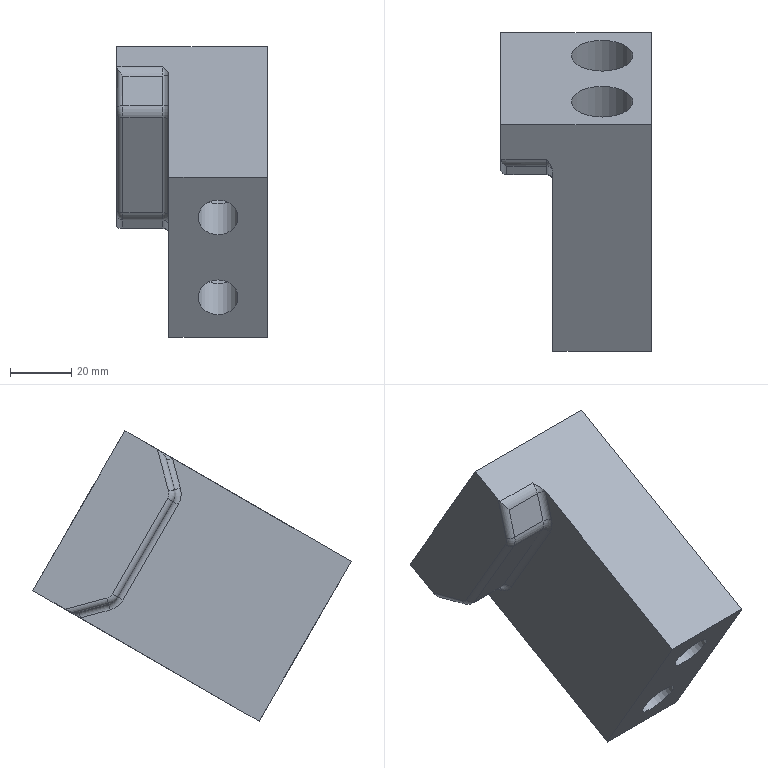Part | NX | features solid 2 | 1 solid | 32 faces | box 49 x 103.612 x 94.462 mm | volume 140816 mm3 | cylinder 14 | plane 12 | torus 6 | commonest cylinder face diameters 4 x6 10 x4 13 x2 20 x2
STEP:
#1=CARTESIAN_POINT('',(679.,-646.197,-54.503));
#2=VERTEX_POINT('',#1);
#3=CARTESIAN_POINT('',(664.073,-646.197,-54.503));
#4=VERTEX_POINT('',#3);
#5=CARTESIAN_POINT('',(713.,-646.197,-54.503));
#6=DIRECTION('',(-1.,0.,0.));
#7=VECTOR('',#6,1000.);
#8=LINE('',#5,#7);
#9=EDGE_CURVE('',#2,#4,#8,.T.);
#10=ORIENTED_EDGE('',*,*,#9,.T.);
#11=CARTESIAN_POINT('',(664.,-645.541,-54.124));
#12=VERTEX_POINT('',#11);
#13=CARTESIAN_POINT('',(666.,-645.541,-54.124));
#14=DIRECTION('',(0.,0.5,-0.866));
#15=DIRECTION('',(0.,-0.866,-0.5));
#16=AXIS2_PLACEMENT_3D('',#13,#14,#15);
#17=ELLIPSE('',#16,2.828,2.);
#18=EDGE_CURVE('',#4,#12,#17,.T.);
#19=ORIENTED_EDGE('',*,*,#18,.T.);
#20=CARTESIAN_POINT('',(664.,-635.,-48.038));
#21=VERTEX_POINT('',#20);
#22=CARTESIAN_POINT('',(664.,-635.,-48.038));
#23=DIRECTION('',(0.,-0.866,-0.5));
#24=VECTOR('',#23,1000.);
#25=LINE('',#22,#24);
#26=EDGE_CURVE('',#21,#12,#25,.T.);
#27=ORIENTED_EDGE('',*,*,#26,.F.);
#28=CARTESIAN_POINT('',(713.,-635.,-48.038));
#29=VERTEX_POINT('',#28);
#30=CARTESIAN_POINT('',(713.,-635.,-48.038));
#31=DIRECTION('',(-1.,0.,0.));
#32=VECTOR('',#31,1000.);
#33=LINE('',#30,#32);
#34=EDGE_CURVE('',#29,#21,#33,.T.);
#35=ORIENTED_EDGE('',*,*,#34,.F.);
#36=CARTESIAN_POINT('',(713.,-708.612,-90.538));
#37=VERTEX_POINT('',#36);
#38=CARTESIAN_POINT('',(713.,-635.,-48.038));
#39=DIRECTION('',(0.,-0.866,-0.5));
#40=VECTOR('',#39,1000.);
#41=LINE('',#38,#40);
#42=EDGE_CURVE('',#29,#37,#41,.T.);
#43=ORIENTED_EDGE('',*,*,#42,.T.);
#44=CARTESIAN_POINT('',(681.,-708.612,-90.538));
#45=VERTEX_POINT('',#44);
#46=CARTESIAN_POINT('',(713.,-708.612,-90.538));
#47=DIRECTION('',(-1.,0.,0.));
#48=VECTOR('',#47,1000.);
#49=LINE('',#46,#48);
#50=EDGE_CURVE('',#37,#45,#49,.T.);
#51=ORIENTED_EDGE('',*,*,#50,.T.);
#52=CARTESIAN_POINT('',(681.,-650.439,-56.952));
#53=VERTEX_POINT('',#52);
#54=CARTESIAN_POINT('',(681.,-656.651,-60.538));
#55=DIRECTION('',(0.,-0.866,-0.5));
#56=VECTOR('',#55,1000.);
#57=LINE('',#54,#56);
#58=EDGE_CURVE('',#53,#45,#57,.T.);
#59=ORIENTED_EDGE('',*,*,#58,.F.);
#60=CARTESIAN_POINT('',(681.,-650.439,-56.952));
#61=CARTESIAN_POINT('',(681.,-649.654,-56.499));
#62=CARTESIAN_POINT('',(680.429,-648.15,-55.631));
#63=CARTESIAN_POINT('',(679.478,-646.851,-54.881));
#64=CARTESIAN_POINT('',(679.,-646.197,-54.503));
#65=B_SPLINE_CURVE_WITH_KNOTS('',3,(#60,#61,#62,#63,#64),.UNSPECIFIED.,.F.,.F.,(4,1,4),(0.,0.002683,0.005365),.UNSPECIFIED.);
#66=EDGE_CURVE('',#53,#2,#65,.T.);
#67=ORIENTED_EDGE('',*,*,#66,.T.);
#68=EDGE_LOOP('',(#10,#19,#27,#35,#43,#51,#59,#67));
#69=FACE_BOUND('',#68,.T.);
#70=CARTESIAN_POINT('',(713.,-635.,-48.038));
#71=DIRECTION('',(0.,0.5,-0.866));
#72=DIRECTION('',(-0.2144,-0.8459,-0.4884));
#73=AXIS2_PLACEMENT_3D('',#70,#71,#72);
#74=PLANE('',#73);
#75=ADVANCED_FACE('',(#69),#74,.T.);
#76=CARTESIAN_POINT('',(697.,-727.862,-57.196));
#77=VERTEX_POINT('',#76);
#78=CARTESIAN_POINT('',(697.,-731.112,-51.567));
#79=DIRECTION('',(0.,-0.866,-0.5));
#80=DIRECTION('',(0.,0.5,-0.866));
#81=AXIS2_PLACEMENT_3D('',#78,#79,#80);
#82=CIRCLE('',#81,6.5);
#83=EDGE_CURVE('',#77,#77,#82,.T.);
#84=ORIENTED_EDGE('',*,*,#83,.F.);
#85=EDGE_LOOP('',(#84));
#86=FACE_BOUND('',#85,.T.);
#87=CARTESIAN_POINT('',(697.,-712.862,-83.177));
#88=VERTEX_POINT('',#87);
#89=CARTESIAN_POINT('',(697.,-716.112,-77.548));
#90=DIRECTION('',(0.,-0.866,-0.5));
#91=DIRECTION('',(0.,0.5,-0.866));
#92=AXIS2_PLACEMENT_3D('',#89,#90,#91);
#93=CIRCLE('',#92,6.5);
#94=EDGE_CURVE('',#88,#88,#93,.T.);
#95=ORIENTED_EDGE('',*,*,#94,.F.);
#96=EDGE_LOOP('',(#95));
#97=FACE_BOUND('',#96,.T.);
#98=CARTESIAN_POINT('',(713.,-738.612,-38.577));
#99=VERTEX_POINT('',#98);
#100=CARTESIAN_POINT('',(681.,-738.612,-38.577));
#101=VERTEX_POINT('',#100);
#102=CARTESIAN_POINT('',(713.,-738.612,-38.577));
#103=DIRECTION('',(-1.,0.,0.));
#104=VECTOR('',#103,1000.);
#105=LINE('',#102,#104);
#106=EDGE_CURVE('',#99,#101,#105,.T.);
#107=ORIENTED_EDGE('',*,*,#106,.T.);
#108=CARTESIAN_POINT('',(681.,-738.612,-38.577));
#109=DIRECTION('',(0.,0.5,-0.866));
#110=VECTOR('',#109,1000.);
#111=LINE('',#108,#110);
#112=EDGE_CURVE('',#101,#45,#111,.T.);
#113=ORIENTED_EDGE('',*,*,#112,.T.);
#114=ORIENTED_EDGE('',*,*,#50,.F.);
#115=CARTESIAN_POINT('',(713.,-761.112,0.3942));
#116=DIRECTION('',(0.,0.5,-0.866));
#117=VECTOR('',#116,1000.);
#118=LINE('',#115,#117);
#119=EDGE_CURVE('',#99,#37,#118,.T.);
#120=ORIENTED_EDGE('',*,*,#119,.F.);
#121=EDGE_LOOP('',(#107,#113,#114,#120));
#122=FACE_BOUND('',#121,.T.);
#123=CARTESIAN_POINT('',(713.,-761.112,0.3942));
#124=DIRECTION('',(0.,0.866,0.5));
#125=DIRECTION('',(-0.1519,0.4942,-0.856));
#126=AXIS2_PLACEMENT_3D('',#123,#124,#125);
#127=PLANE('',#126);
#128=ADVANCED_FACE('',(#86,#97,#122),#127,.F.);
#129=CARTESIAN_POINT('',(664.,-665.,3.923));
#130=VERTEX_POINT('',#129);
#131=CARTESIAN_POINT('',(664.,-675.541,-2.163));
#132=VERTEX_POINT('',#131);
#133=CARTESIAN_POINT('',(664.,-665.,3.923));
#134=DIRECTION('',(0.,-0.866,-0.5));
#135=VECTOR('',#134,1000.);
#136=LINE('',#133,#135);
#137=EDGE_CURVE('',#130,#132,#136,.T.);
#138=ORIENTED_EDGE('',*,*,#137,.T.);
#139=CARTESIAN_POINT('',(664.073,-676.197,-2.541));
#140=VERTEX_POINT('',#139);
#141=CARTESIAN_POINT('',(666.,-675.541,-2.163));
#142=DIRECTION('',(0.,-0.5,0.866));
#143=DIRECTION('',(0.,-0.866,-0.5));
#144=AXIS2_PLACEMENT_3D('',#141,#142,#143);
#145=ELLIPSE('',#144,2.828,2.);
#146=EDGE_CURVE('',#132,#140,#145,.T.);
#147=ORIENTED_EDGE('',*,*,#146,.T.);
#148=CARTESIAN_POINT('',(679.,-676.197,-2.541));
#149=VERTEX_POINT('',#148);
#150=CARTESIAN_POINT('',(713.,-676.197,-2.541));
#151=DIRECTION('',(1.,0.,0.));
#152=VECTOR('',#151,1000.);
#153=LINE('',#150,#152);
#154=EDGE_CURVE('',#140,#149,#153,.T.);
#155=ORIENTED_EDGE('',*,*,#154,.T.);
#156=CARTESIAN_POINT('',(681.,-680.439,-4.991));
#157=VERTEX_POINT('',#156);
#158=CARTESIAN_POINT('',(679.,-676.197,-2.541));
#159=CARTESIAN_POINT('',(679.475,-676.847,-2.917));
#160=CARTESIAN_POINT('',(680.428,-678.147,-3.668));
#161=CARTESIAN_POINT('',(681.,-679.656,-4.539));
#162=CARTESIAN_POINT('',(681.,-680.439,-4.991));
#163=B_SPLINE_CURVE_WITH_KNOTS('',3,(#158,#159,#160,#161,#162),.UNSPECIFIED.,.F.,.F.,(4,1,4),(-0.00001414,0.002651,0.005315),.UNSPECIFIED.);
#164=EDGE_CURVE('',#149,#157,#163,.T.);
#165=ORIENTED_EDGE('',*,*,#164,.T.);
#166=CARTESIAN_POINT('',(681.,-686.651,-8.577));
#167=DIRECTION('',(0.,-0.866,-0.5));
#168=VECTOR('',#167,1000.);
#169=LINE('',#166,#168);
#170=EDGE_CURVE('',#157,#101,#169,.T.);
#171=ORIENTED_EDGE('',*,*,#170,.T.);
#172=ORIENTED_EDGE('',*,*,#106,.F.);
#173=CARTESIAN_POINT('',(713.,-665.,3.923));
#174=VERTEX_POINT('',#173);
#175=CARTESIAN_POINT('',(713.,-665.,3.923));
#176=DIRECTION('',(0.,-0.866,-0.5));
#177=VECTOR('',#176,1000.);
#178=LINE('',#175,#177);
#179=EDGE_CURVE('',#174,#99,#178,.T.);
#180=ORIENTED_EDGE('',*,*,#179,.F.);
#181=CARTESIAN_POINT('',(713.,-665.,3.923));
#182=DIRECTION('',(-1.,0.,0.));
#183=VECTOR('',#182,1000.);
#184=LINE('',#181,#183);
#185=EDGE_CURVE('',#174,#130,#184,.T.);
#186=ORIENTED_EDGE('',*,*,#185,.T.);
#187=EDGE_LOOP('',(#138,#147,#155,#165,#171,#172,#180,#186));
#188=FACE_BOUND('',#187,.T.);
#189=CARTESIAN_POINT('',(713.,-665.,3.923));
#190=DIRECTION('',(0.,0.5,-0.866));
#191=DIRECTION('',(-0.2144,-0.8459,-0.4884));
#192=AXIS2_PLACEMENT_3D('',#189,#190,#191);
#193=PLANE('',#192);
#194=ADVANCED_FACE('',(#188),#193,.F.);
#195=CARTESIAN_POINT('',(664.,-678.883,-18.031));
#196=VERTEX_POINT('',#195);
#197=CARTESIAN_POINT('',(664.,-679.183,-15.754));
#198=VERTEX_POINT('',#197);
#199=CARTESIAN_POINT('',(664.,-676.285,-16.531));
#200=DIRECTION('',(-1.,0.,0.));
#201=DIRECTION('',(0.,-0.866,0.5));
#202=AXIS2_PLACEMENT_3D('',#199,#200,#201);
#203=CIRCLE('',#202,3.);
#204=EDGE_CURVE('',#196,#198,#203,.T.);
#205=ORIENTED_EDGE('',*,*,#204,.T.);
#206=CARTESIAN_POINT('',(664.,-665.078,36.886));
#207=DIRECTION('',(0.,0.2588,0.9659));
#208=VECTOR('',#207,1000.);
#209=LINE('',#206,#208);
#210=EDGE_CURVE('',#198,#132,#209,.T.);
#211=ORIENTED_EDGE('',*,*,#210,.T.);
#212=ORIENTED_EDGE('',*,*,#137,.F.);
#213=CARTESIAN_POINT('',(664.,-687.5,42.894));
#214=DIRECTION('',(0.,0.5,-0.866));
#215=VECTOR('',#214,1000.);
#216=LINE('',#213,#215);
#217=EDGE_CURVE('',#130,#21,#216,.T.);
#218=ORIENTED_EDGE('',*,*,#217,.T.);
#219=ORIENTED_EDGE('',*,*,#26,.T.);
#220=CARTESIAN_POINT('',(664.,-659.132,-50.482));
#221=VERTEX_POINT('',#220);
#222=CARTESIAN_POINT('',(664.,-708.944,-37.135));
#223=DIRECTION('',(0.,-0.9659,0.2588));
#224=VECTOR('',#223,1000.);
#225=LINE('',#222,#224);
#226=EDGE_CURVE('',#12,#221,#225,.T.);
#227=ORIENTED_EDGE('',*,*,#226,.T.);
#228=CARTESIAN_POINT('',(664.,-660.954,-49.085));
#229=VERTEX_POINT('',#228);
#230=CARTESIAN_POINT('',(664.,-658.356,-47.585));
#231=DIRECTION('',(-1.,0.,0.));
#232=DIRECTION('',(0.,-0.866,0.5));
#233=AXIS2_PLACEMENT_3D('',#230,#231,#232);
#234=CIRCLE('',#233,3.);
#235=EDGE_CURVE('',#221,#229,#234,.T.);
#236=ORIENTED_EDGE('',*,*,#235,.T.);
#237=CARTESIAN_POINT('',(664.,-707.419,31.394));
#238=DIRECTION('',(0.,-0.5,0.866));
#239=VECTOR('',#238,1000.);
#240=LINE('',#237,#239);
#241=EDGE_CURVE('',#229,#196,#240,.T.);
#242=ORIENTED_EDGE('',*,*,#241,.T.);
#243=EDGE_LOOP('',(#205,#211,#212,#218,#219,#227,#236,#242));
#244=FACE_BOUND('',#243,.T.);
#245=CARTESIAN_POINT('',(664.,-687.5,42.894));
#246=DIRECTION('',(-1.,0.,0.));
#247=DIRECTION('',(0.,0.4226,0.9063));
#248=AXIS2_PLACEMENT_3D('',#245,#246,#247);
#249=PLANE('',#248);
#250=ADVANCED_FACE('',(#244),#249,.T.);
#251=CARTESIAN_POINT('',(697.,-662.5,-0.4071));
#252=VERTEX_POINT('',#251);
#253=CARTESIAN_POINT('',(697.,-657.5,-9.067));
#254=DIRECTION('',(0.,-0.866,-0.5));
#255=DIRECTION('',(0.,-0.5,0.866));
#256=AXIS2_PLACEMENT_3D('',#253,#254,#255);
#257=CIRCLE('',#256,10.);
#258=EDGE_CURVE('',#252,#252,#257,.T.);
#259=ORIENTED_EDGE('',*,*,#258,.T.);
#260=EDGE_LOOP('',(#259));
#261=FACE_BOUND('',#260,.T.);
#262=CARTESIAN_POINT('',(697.,-647.5,-26.388));
#263=VERTEX_POINT('',#262);
#264=CARTESIAN_POINT('',(697.,-642.5,-35.048));
#265=DIRECTION('',(0.,-0.866,-0.5));
#266=DIRECTION('',(0.,-0.5,0.866));
#267=AXIS2_PLACEMENT_3D('',#264,#265,#266);
#268=CIRCLE('',#267,10.);
#269=EDGE_CURVE('',#263,#263,#268,.T.);
#270=ORIENTED_EDGE('',*,*,#269,.T.);
#271=EDGE_LOOP('',(#270));
#272=FACE_BOUND('',#271,.T.);
#273=ORIENTED_EDGE('',*,*,#185,.F.);
#274=CARTESIAN_POINT('',(713.,-687.5,42.894));
#275=DIRECTION('',(0.,0.5,-0.866));
#276=VECTOR('',#275,1000.);
#277=LINE('',#274,#276);
#278=EDGE_CURVE('',#174,#29,#277,.T.);
#279=ORIENTED_EDGE('',*,*,#278,.T.);
#280=ORIENTED_EDGE('',*,*,#34,.T.);
#281=ORIENTED_EDGE('',*,*,#217,.F.);
#282=EDGE_LOOP('',(#273,#279,#280,#281));
#283=FACE_BOUND('',#282,.T.);
#284=CARTESIAN_POINT('',(713.,-687.5,42.894));
#285=DIRECTION('',(0.,0.866,0.5));
#286=DIRECTION('',(-0.1519,0.4942,-0.856));
#287=AXIS2_PLACEMENT_3D('',#284,#285,#286);
#288=PLANE('',#287);
#289=ADVANCED_FACE('',(#261,#272,#283),#288,.T.);
#290=ORIENTED_EDGE('',*,*,#119,.T.);
#291=ORIENTED_EDGE('',*,*,#42,.F.);
#292=ORIENTED_EDGE('',*,*,#278,.F.);
#293=ORIENTED_EDGE('',*,*,#179,.T.);
#294=EDGE_LOOP('',(#290,#291,#292,#293));
#295=FACE_BOUND('',#294,.T.);
#296=CARTESIAN_POINT('',(713.,-687.5,42.894));
#297=DIRECTION('',(-1.,0.,0.));
#298=DIRECTION('',(0.,0.4226,0.9063));
#299=AXIS2_PLACEMENT_3D('',#296,#297,#298);
#300=PLANE('',#299);
#301=ADVANCED_FACE('',(#295),#300,.F.);
#302=CARTESIAN_POINT('',(679.,-680.615,-19.031));
#303=VERTEX_POINT('',#302);
#304=CARTESIAN_POINT('',(666.,-680.615,-19.031));
#305=VERTEX_POINT('',#304);
#306=CARTESIAN_POINT('',(713.,-680.615,-19.031));
#307=DIRECTION('',(-1.,0.,0.));
#308=VECTOR('',#307,1000.);
#309=LINE('',#306,#308);
#310=EDGE_CURVE('',#303,#305,#309,.T.);
#311=ORIENTED_EDGE('',*,*,#310,.T.);
#312=CARTESIAN_POINT('',(666.,-662.686,-50.085));
#313=VERTEX_POINT('',#312);
#314=CARTESIAN_POINT('',(666.,-686.651,-8.577));
#315=DIRECTION('',(0.,0.5,-0.866));
#316=VECTOR('',#315,1000.);
#317=LINE('',#314,#316);
#318=EDGE_CURVE('',#305,#313,#317,.T.);
#319=ORIENTED_EDGE('',*,*,#318,.T.);
#320=CARTESIAN_POINT('',(679.,-662.686,-50.085));
#321=VERTEX_POINT('',#320);
#322=CARTESIAN_POINT('',(713.,-662.686,-50.085));
#323=DIRECTION('',(1.,0.,0.));
#324=VECTOR('',#323,1000.);
#325=LINE('',#322,#324);
#326=EDGE_CURVE('',#313,#321,#325,.T.);
#327=ORIENTED_EDGE('',*,*,#326,.T.);
#328=CARTESIAN_POINT('',(679.,-680.615,-19.031));
#329=DIRECTION('',(0.,-0.5,0.866));
#330=VECTOR('',#329,1000.);
#331=LINE('',#328,#330);
#332=EDGE_CURVE('',#321,#303,#331,.T.);
#333=ORIENTED_EDGE('',*,*,#332,.T.);
#334=EDGE_LOOP('',(#311,#319,#327,#333));
#335=FACE_BOUND('',#334,.T.);
#336=CARTESIAN_POINT('',(713.,-686.651,-8.577));
#337=DIRECTION('',(0.,0.866,0.5));
#338=DIRECTION('',(-0.1519,0.4942,-0.856));
#339=AXIS2_PLACEMENT_3D('',#336,#337,#338);
#340=PLANE('',#339);
#341=ADVANCED_FACE('',(#335),#340,.F.);
#342=ORIENTED_EDGE('',*,*,#170,.F.);
#343=CARTESIAN_POINT('',(681.,-680.458,-5.06));
#344=VERTEX_POINT('',#343);
#345=CARTESIAN_POINT('',(681.,-673.697,-6.872));
#346=DIRECTION('',(1.,0.,0.));
#347=DIRECTION('',(0.,-0.866,0.5));
#348=AXIS2_PLACEMENT_3D('',#345,#346,#347);
#349=CIRCLE('',#348,7.);
#350=EDGE_CURVE('',#157,#344,#349,.T.);
#351=ORIENTED_EDGE('',*,*,#350,.T.);
#352=CARTESIAN_POINT('',(681.,-683.046,-14.719));
#353=VERTEX_POINT('',#352);
#354=CARTESIAN_POINT('',(681.,-683.046,-14.719));
#355=DIRECTION('',(0.,-0.2588,-0.9659));
#356=VECTOR('',#355,1000.);
#357=LINE('',#354,#356);
#358=EDGE_CURVE('',#344,#353,#357,.T.);
#359=ORIENTED_EDGE('',*,*,#358,.T.);
#360=CARTESIAN_POINT('',(681.,-682.347,-20.031));
#361=VERTEX_POINT('',#360);
#362=CARTESIAN_POINT('',(681.,-676.285,-16.531));
#363=DIRECTION('',(1.,0.,0.));
#364=DIRECTION('',(0.,-0.866,0.5));
#365=AXIS2_PLACEMENT_3D('',#362,#363,#364);
#366=CIRCLE('',#365,7.);
#367=EDGE_CURVE('',#353,#361,#366,.T.);
#368=ORIENTED_EDGE('',*,*,#367,.T.);
#369=CARTESIAN_POINT('',(681.,-664.418,-51.085));
#370=VERTEX_POINT('',#369);
#371=CARTESIAN_POINT('',(681.,-664.418,-51.085));
#372=DIRECTION('',(0.,0.5,-0.866));
#373=VECTOR('',#372,1000.);
#374=LINE('',#371,#373);
#375=EDGE_CURVE('',#361,#370,#374,.T.);
#376=ORIENTED_EDGE('',*,*,#375,.T.);
#377=CARTESIAN_POINT('',(681.,-660.168,-54.346));
#378=VERTEX_POINT('',#377);
#379=CARTESIAN_POINT('',(681.,-658.356,-47.585));
#380=DIRECTION('',(1.,0.,0.));
#381=DIRECTION('',(0.,-0.866,0.5));
#382=AXIS2_PLACEMENT_3D('',#379,#380,#381);
#383=CIRCLE('',#382,7.);
#384=EDGE_CURVE('',#370,#378,#383,.T.);
#385=ORIENTED_EDGE('',*,*,#384,.T.);
#386=CARTESIAN_POINT('',(681.,-650.509,-56.934));
#387=VERTEX_POINT('',#386);
#388=CARTESIAN_POINT('',(681.,-650.509,-56.934));
#389=DIRECTION('',(0.,0.9659,-0.2588));
#390=VECTOR('',#389,1000.);
#391=LINE('',#388,#390);
#392=EDGE_CURVE('',#378,#387,#391,.T.);
#393=ORIENTED_EDGE('',*,*,#392,.T.);
#394=CARTESIAN_POINT('',(681.,-648.697,-50.173));
#395=DIRECTION('',(1.,0.,0.));
#396=DIRECTION('',(0.,-0.866,0.5));
#397=AXIS2_PLACEMENT_3D('',#394,#395,#396);
#398=CIRCLE('',#397,7.);
#399=EDGE_CURVE('',#387,#53,#398,.T.);
#400=ORIENTED_EDGE('',*,*,#399,.T.);
#401=ORIENTED_EDGE('',*,*,#58,.T.);
#402=ORIENTED_EDGE('',*,*,#112,.F.);
#403=EDGE_LOOP('',(#342,#351,#359,#368,#376,#385,#393,#400,#401,#402));
#404=FACE_BOUND('',#403,.T.);
#405=CARTESIAN_POINT('',(681.,-686.651,-8.577));
#406=DIRECTION('',(-1.,0.,0.));
#407=DIRECTION('',(0.,0.4226,0.9063));
#408=AXIS2_PLACEMENT_3D('',#405,#406,#407);
#409=PLANE('',#408);
#410=ADVANCED_FACE('',(#404),#409,.T.);
#411=CARTESIAN_POINT('',(679.,-678.526,-5.577));
#412=VERTEX_POINT('',#411);
#413=CARTESIAN_POINT('',(666.,-678.526,-5.577));
#414=VERTEX_POINT('',#413);
#415=CARTESIAN_POINT('',(713.,-678.526,-5.577));
#416=DIRECTION('',(-1.,0.,0.));
#417=VECTOR('',#416,1000.);
#418=LINE('',#415,#417);
#419=EDGE_CURVE('',#412,#414,#418,.T.);
#420=ORIENTED_EDGE('',*,*,#419,.T.);
#421=CARTESIAN_POINT('',(666.,-681.115,-15.237));
#422=VERTEX_POINT('',#421);
#423=CARTESIAN_POINT('',(666.,-677.99,-3.577));
#424=DIRECTION('',(0.,-0.2588,-0.9659));
#425=VECTOR('',#424,1000.);
#426=LINE('',#423,#425);
#427=EDGE_CURVE('',#414,#422,#426,.T.);
#428=ORIENTED_EDGE('',*,*,#427,.T.);
#429=CARTESIAN_POINT('',(679.,-681.115,-15.237));
#430=VERTEX_POINT('',#429);
#431=CARTESIAN_POINT('',(713.,-681.115,-15.237));
#432=DIRECTION('',(1.,0.,0.));
#433=VECTOR('',#432,1000.);
#434=LINE('',#431,#433);
#435=EDGE_CURVE('',#422,#430,#434,.T.);
#436=ORIENTED_EDGE('',*,*,#435,.T.);
#437=CARTESIAN_POINT('',(679.,-678.526,-5.577));
#438=DIRECTION('',(0.,0.2588,0.9659));
#439=VECTOR('',#438,1000.);
#440=LINE('',#437,#439);
#441=EDGE_CURVE('',#430,#412,#440,.T.);
#442=ORIENTED_EDGE('',*,*,#441,.T.);
#443=EDGE_LOOP('',(#420,#428,#436,#442));
#444=FACE_BOUND('',#443,.T.);
#445=CARTESIAN_POINT('',(713.,-677.99,-3.577));
#446=DIRECTION('',(0.,0.9659,-0.2588));
#447=DIRECTION('',(-0.2551,-0.2503,-0.934));
#448=AXIS2_PLACEMENT_3D('',#445,#446,#447);
#449=PLANE('',#448);
#450=ADVANCED_FACE('',(#444),#449,.F.);
#451=CARTESIAN_POINT('',(679.,-659.65,-52.414));
#452=VERTEX_POINT('',#451);
#453=CARTESIAN_POINT('',(666.,-659.65,-52.414));
#454=VERTEX_POINT('',#453);
#455=CARTESIAN_POINT('',(713.,-659.65,-52.414));
#456=DIRECTION('',(-1.,0.,0.));
#457=VECTOR('',#456,1000.);
#458=LINE('',#455,#457);
#459=EDGE_CURVE('',#452,#454,#458,.T.);
#460=ORIENTED_EDGE('',*,*,#459,.T.);
#461=CARTESIAN_POINT('',(666.,-649.991,-55.002));
#462=VERTEX_POINT('',#461);
#463=CARTESIAN_POINT('',(666.,-661.651,-51.878));
#464=DIRECTION('',(0.,0.9659,-0.2588));
#465=VECTOR('',#464,1000.);
#466=LINE('',#463,#465);
#467=EDGE_CURVE('',#454,#462,#466,.T.);
#468=ORIENTED_EDGE('',*,*,#467,.T.);
#469=CARTESIAN_POINT('',(679.,-649.991,-55.002));
#470=VERTEX_POINT('',#469);
#471=CARTESIAN_POINT('',(713.,-649.991,-55.002));
#472=DIRECTION('',(1.,0.,0.));
#473=VECTOR('',#472,1000.);
#474=LINE('',#471,#473);
#475=EDGE_CURVE('',#462,#470,#474,.T.);
#476=ORIENTED_EDGE('',*,*,#475,.T.);
#477=CARTESIAN_POINT('',(679.,-659.65,-52.414));
#478=DIRECTION('',(0.,-0.9659,0.2588));
#479=VECTOR('',#478,1000.);
#480=LINE('',#477,#479);
#481=EDGE_CURVE('',#470,#452,#480,.T.);
#482=ORIENTED_EDGE('',*,*,#481,.T.);
#483=EDGE_LOOP('',(#460,#468,#476,#482));
#484=FACE_BOUND('',#483,.T.);
#485=CARTESIAN_POINT('',(713.,-661.651,-51.878));
#486=DIRECTION('',(0.,-0.2588,-0.9659));
#487=DIRECTION('',(-1.,0.,0.));
#488=AXIS2_PLACEMENT_3D('',#485,#486,#487);
#489=PLANE('',#488);
#490=ADVANCED_FACE('',(#484),#489,.T.);
#491=ORIENTED_EDGE('',*,*,#475,.F.);
#492=CARTESIAN_POINT('',(666.,-649.991,-55.002));
#493=CARTESIAN_POINT('',(665.22,-648.8,-55.322));
#494=CARTESIAN_POINT('',(664.356,-647.444,-55.223));
#495=CARTESIAN_POINT('',(664.073,-646.197,-54.503));
#496=B_SPLINE_CURVE_WITH_KNOTS('',3,(#492,#493,#494,#495),.UNSPECIFIED.,.F.,.F.,(4,4),(-0.00001414,0.004362),.UNSPECIFIED.);
#497=EDGE_CURVE('',#462,#4,#496,.T.);
#498=ORIENTED_EDGE('',*,*,#497,.T.);
#499=ORIENTED_EDGE('',*,*,#9,.F.);
#500=CARTESIAN_POINT('',(679.,-648.697,-50.173));
#501=DIRECTION('',(-1.,0.,0.));
#502=DIRECTION('',(0.,-0.866,0.5));
#503=AXIS2_PLACEMENT_3D('',#500,#501,#502);
#504=CIRCLE('',#503,5.);
#505=EDGE_CURVE('',#2,#470,#504,.T.);
#506=ORIENTED_EDGE('',*,*,#505,.T.);
#507=EDGE_LOOP('',(#491,#498,#499,#506));
#508=FACE_BOUND('',#507,.T.);
#509=CARTESIAN_POINT('',(713.,-648.697,-50.173));
#510=DIRECTION('',(-1.,0.,0.));
#511=DIRECTION('',(0.,0.4226,0.9063));
#512=AXIS2_PLACEMENT_3D('',#509,#510,#511);
#513=CYLINDRICAL_SURFACE('',#512,5.);
#514=ADVANCED_FACE('',(#508),#513,.T.);
#515=ORIENTED_EDGE('',*,*,#326,.F.);
#516=CARTESIAN_POINT('',(666.,-658.356,-47.585));
#517=DIRECTION('',(1.,0.,0.));
#518=DIRECTION('',(0.,-0.866,0.5));
#519=AXIS2_PLACEMENT_3D('',#516,#517,#518);
#520=CIRCLE('',#519,5.);
#521=EDGE_CURVE('',#313,#454,#520,.T.);
#522=ORIENTED_EDGE('',*,*,#521,.T.);
#523=ORIENTED_EDGE('',*,*,#459,.F.);
#524=CARTESIAN_POINT('',(679.,-658.356,-47.585));
#525=DIRECTION('',(-1.,0.,0.));
#526=DIRECTION('',(0.,-0.866,0.5));
#527=AXIS2_PLACEMENT_3D('',#524,#525,#526);
#528=CIRCLE('',#527,5.);
#529=EDGE_CURVE('',#452,#321,#528,.T.);
#530=ORIENTED_EDGE('',*,*,#529,.T.);
#531=EDGE_LOOP('',(#515,#522,#523,#530));
#532=FACE_BOUND('',#531,.T.);
#533=CARTESIAN_POINT('',(713.,-658.356,-47.585));
#534=DIRECTION('',(-1.,0.,0.));
#535=DIRECTION('',(0.,0.4226,0.9063));
#536=AXIS2_PLACEMENT_3D('',#533,#534,#535);
#537=CYLINDRICAL_SURFACE('',#536,5.);
#538=ADVANCED_FACE('',(#532),#537,.T.);
#539=ORIENTED_EDGE('',*,*,#435,.F.);
#540=CARTESIAN_POINT('',(666.,-676.285,-16.531));
#541=DIRECTION('',(1.,0.,0.));
#542=DIRECTION('',(0.,-0.866,0.5));
#543=AXIS2_PLACEMENT_3D('',#540,#541,#542);
#544=CIRCLE('',#543,5.);
#545=EDGE_CURVE('',#422,#305,#544,.T.);
#546=ORIENTED_EDGE('',*,*,#545,.T.);
#547=ORIENTED_EDGE('',*,*,#310,.F.);
#548=CARTESIAN_POINT('',(679.,-676.285,-16.531));
#549=DIRECTION('',(-1.,0.,0.));
#550=DIRECTION('',(0.,-0.866,0.5));
#551=AXIS2_PLACEMENT_3D('',#548,#549,#550);
#552=CIRCLE('',#551,5.);
#553=EDGE_CURVE('',#303,#430,#552,.T.);
#554=ORIENTED_EDGE('',*,*,#553,.T.);
#555=EDGE_LOOP('',(#539,#546,#547,#554));
#556=FACE_BOUND('',#555,.T.);
#557=CARTESIAN_POINT('',(713.,-676.285,-16.531));
#558=DIRECTION('',(-1.,0.,0.));
#559=DIRECTION('',(0.,0.4226,0.9063));
#560=AXIS2_PLACEMENT_3D('',#557,#558,#559);
#561=CYLINDRICAL_SURFACE('',#560,5.);
#562=ADVANCED_FACE('',(#556),#561,.T.);
#563=ORIENTED_EDGE('',*,*,#154,.F.);
#564=CARTESIAN_POINT('',(664.073,-676.197,-2.541));
#565=CARTESIAN_POINT('',(664.359,-677.457,-3.269));
#566=CARTESIAN_POINT('',(665.219,-678.207,-4.385));
#567=CARTESIAN_POINT('',(666.,-678.526,-5.577));
#568=B_SPLINE_CURVE_WITH_KNOTS('',3,(#564,#565,#566,#567),.UNSPECIFIED.,.F.,.F.,(4,4),(0.,0.004383),.UNSPECIFIED.);
#569=EDGE_CURVE('',#140,#414,#568,.T.);
#570=ORIENTED_EDGE('',*,*,#569,.T.);
#571=ORIENTED_EDGE('',*,*,#419,.F.);
#572=CARTESIAN_POINT('',(679.,-673.697,-6.872));
#573=DIRECTION('',(-1.,0.,0.));
#574=DIRECTION('',(0.,-0.866,0.5));
#575=AXIS2_PLACEMENT_3D('',#572,#573,#574);
#576=CIRCLE('',#575,5.);
#577=EDGE_CURVE('',#412,#149,#576,.T.);
#578=ORIENTED_EDGE('',*,*,#577,.T.);
#579=EDGE_LOOP('',(#563,#570,#571,#578));
#580=FACE_BOUND('',#579,.T.);
#581=CARTESIAN_POINT('',(713.,-673.697,-6.872));
#582=DIRECTION('',(1.,0.,0.));
#583=DIRECTION('',(0.,-0.4226,-0.9063));
#584=AXIS2_PLACEMENT_3D('',#581,#582,#583);
#585=CYLINDRICAL_SURFACE('',#584,5.);
#586=ADVANCED_FACE('',(#580),#585,.T.);
#587=ORIENTED_EDGE('',*,*,#66,.F.);
#588=ORIENTED_EDGE('',*,*,#399,.F.);
#589=CARTESIAN_POINT('',(679.,-650.509,-56.934));
#590=DIRECTION('',(0.,0.9659,-0.2588));
#591=DIRECTION('',(0.,-0.2588,-0.9659));
#592=AXIS2_PLACEMENT_3D('',#589,#590,#591);
#593=CIRCLE('',#592,2.);
#594=EDGE_CURVE('',#470,#387,#593,.T.);
#595=ORIENTED_EDGE('',*,*,#594,.F.);
#596=ORIENTED_EDGE('',*,*,#505,.F.);
#597=EDGE_LOOP('',(#587,#588,#595,#596));
#598=FACE_BOUND('',#597,.T.);
#599=CARTESIAN_POINT('',(679.,-648.697,-50.173));
#600=DIRECTION('',(-1.,0.,0.));
#601=DIRECTION('',(0.,0.4226,0.9063));
#602=AXIS2_PLACEMENT_3D('',#599,#600,#601);
#603=TOROIDAL_SURFACE('',#602,7.,2.);
#604=ADVANCED_FACE('',(#598),#603,.F.);
#605=ORIENTED_EDGE('',*,*,#594,.T.);
#606=ORIENTED_EDGE('',*,*,#392,.F.);
#607=CARTESIAN_POINT('',(679.,-660.168,-54.346));
#608=DIRECTION('',(0.,0.9659,-0.2588));
#609=DIRECTION('',(0.,-0.2588,-0.9659));
#610=AXIS2_PLACEMENT_3D('',#607,#608,#609);
#611=CIRCLE('',#610,2.);
#612=EDGE_CURVE('',#452,#378,#611,.T.);
#613=ORIENTED_EDGE('',*,*,#612,.F.);
#614=ORIENTED_EDGE('',*,*,#481,.F.);
#615=EDGE_LOOP('',(#605,#606,#613,#614));
#616=FACE_BOUND('',#615,.T.);
#617=CARTESIAN_POINT('',(679.,-696.319,-44.659));
#618=DIRECTION('',(0.,-0.9659,0.2588));
#619=DIRECTION('',(0.2551,0.2503,0.934));
#620=AXIS2_PLACEMENT_3D('',#617,#618,#619);
#621=CYLINDRICAL_SURFACE('',#620,2.);
#622=ADVANCED_FACE('',(#616),#621,.F.);
#623=ORIENTED_EDGE('',*,*,#612,.T.);
#624=ORIENTED_EDGE('',*,*,#384,.F.);
#625=CARTESIAN_POINT('',(679.,-664.418,-51.085));
#626=DIRECTION('',(0.,0.5,-0.866));
#627=DIRECTION('',(0.,-0.866,-0.5));
#628=AXIS2_PLACEMENT_3D('',#625,#626,#627);
#629=CIRCLE('',#628,2.);
#630=EDGE_CURVE('',#321,#370,#629,.T.);
#631=ORIENTED_EDGE('',*,*,#630,.F.);
#632=ORIENTED_EDGE('',*,*,#529,.F.);
#633=EDGE_LOOP('',(#623,#624,#631,#632));
#634=FACE_BOUND('',#633,.T.);
#635=CARTESIAN_POINT('',(679.,-658.356,-47.585));
#636=DIRECTION('',(-1.,0.,0.));
#637=DIRECTION('',(0.,0.4226,0.9063));
#638=AXIS2_PLACEMENT_3D('',#635,#636,#637);
#639=TOROIDAL_SURFACE('',#638,7.,2.);
#640=ADVANCED_FACE('',(#634),#639,.F.);
#641=ORIENTED_EDGE('',*,*,#630,.T.);
#642=ORIENTED_EDGE('',*,*,#375,.F.);
#643=CARTESIAN_POINT('',(679.,-682.347,-20.031));
#644=DIRECTION('',(0.,0.5,-0.866));
#645=DIRECTION('',(0.,-0.866,-0.5));
#646=AXIS2_PLACEMENT_3D('',#643,#644,#645);
#647=CIRCLE('',#646,2.);
#648=EDGE_CURVE('',#303,#361,#647,.T.);
#649=ORIENTED_EDGE('',*,*,#648,.F.);
#650=ORIENTED_EDGE('',*,*,#332,.F.);
#651=EDGE_LOOP('',(#641,#642,#649,#650));
#652=FACE_BOUND('',#651,.T.);
#653=CARTESIAN_POINT('',(679.,-688.383,-9.577));
#654=DIRECTION('',(0.,0.5,-0.866));
#655=DIRECTION('',(-0.2144,-0.8459,-0.4884));
#656=AXIS2_PLACEMENT_3D('',#653,#654,#655);
#657=CYLINDRICAL_SURFACE('',#656,2.);
#658=ADVANCED_FACE('',(#652),#657,.F.);
#659=ORIENTED_EDGE('',*,*,#648,.T.);
#660=ORIENTED_EDGE('',*,*,#367,.F.);
#661=CARTESIAN_POINT('',(679.,-683.046,-14.719));
#662=DIRECTION('',(0.,-0.2588,-0.9659));
#663=DIRECTION('',(0.,-0.9659,0.2588));
#664=AXIS2_PLACEMENT_3D('',#661,#662,#663);
#665=CIRCLE('',#664,2.);
#666=EDGE_CURVE('',#430,#353,#665,.T.);
#667=ORIENTED_EDGE('',*,*,#666,.F.);
#668=ORIENTED_EDGE('',*,*,#553,.F.);
#669=EDGE_LOOP('',(#659,#660,#667,#668));
#670=FACE_BOUND('',#669,.T.);
#671=CARTESIAN_POINT('',(679.,-676.285,-16.531));
#672=DIRECTION('',(-1.,0.,0.));
#673=DIRECTION('',(0.,0.4226,0.9063));
#674=AXIS2_PLACEMENT_3D('',#671,#672,#673);
#675=TOROIDAL_SURFACE('',#674,7.,2.);
#676=ADVANCED_FACE('',(#670),#675,.F.);
#677=ORIENTED_EDGE('',*,*,#666,.T.);
#678=ORIENTED_EDGE('',*,*,#358,.F.);
#679=CARTESIAN_POINT('',(679.,-680.458,-5.06));
#680=DIRECTION('',(0.,-0.2588,-0.9659));
#681=DIRECTION('',(0.,-0.9659,0.2588));
#682=AXIS2_PLACEMENT_3D('',#679,#680,#681);
#683=CIRCLE('',#682,2.);
#684=EDGE_CURVE('',#412,#344,#683,.T.);
#685=ORIENTED_EDGE('',*,*,#684,.F.);
#686=ORIENTED_EDGE('',*,*,#441,.F.);
#687=EDGE_LOOP('',(#677,#678,#685,#686));
#688=FACE_BOUND('',#687,.T.);
#689=CARTESIAN_POINT('',(679.,-681.752,-9.889));
#690=DIRECTION('',(0.,-0.2588,-0.9659));
#691=DIRECTION('',(-1.,0.,0.));
#692=AXIS2_PLACEMENT_3D('',#689,#690,#691);
#693=CYLINDRICAL_SURFACE('',#692,2.);
#694=ADVANCED_FACE('',(#688),#693,.F.);
#695=ORIENTED_EDGE('',*,*,#164,.F.);
#696=ORIENTED_EDGE('',*,*,#577,.F.);
#697=ORIENTED_EDGE('',*,*,#684,.T.);
#698=ORIENTED_EDGE('',*,*,#350,.F.);
#699=EDGE_LOOP('',(#695,#696,#697,#698));
#700=FACE_BOUND('',#699,.T.);
#701=CARTESIAN_POINT('',(679.,-673.697,-6.872));
#702=DIRECTION('',(-1.,0.,0.));
#703=DIRECTION('',(0.,0.4226,0.9063));
#704=AXIS2_PLACEMENT_3D('',#701,#702,#703);
#705=TOROIDAL_SURFACE('',#704,7.,2.);
#706=ADVANCED_FACE('',(#700),#705,.F.);
#707=ORIENTED_EDGE('',*,*,#497,.F.);
#708=ORIENTED_EDGE('',*,*,#467,.F.);
#709=CARTESIAN_POINT('',(666.,-659.132,-50.482));
#710=DIRECTION('',(0.,-0.9659,0.2588));
#711=DIRECTION('',(0.,0.2588,0.9659));
#712=AXIS2_PLACEMENT_3D('',#709,#710,#711);
#713=CIRCLE('',#712,2.);
#714=EDGE_CURVE('',#221,#454,#713,.T.);
#715=ORIENTED_EDGE('',*,*,#714,.F.);
#716=ORIENTED_EDGE('',*,*,#226,.F.);
#717=ORIENTED_EDGE('',*,*,#18,.F.);
#718=EDGE_LOOP('',(#707,#708,#715,#716,#717));
#719=FACE_BOUND('',#718,.T.);
#720=CARTESIAN_POINT('',(666.,-708.944,-37.135));
#721=DIRECTION('',(0.,-0.9659,0.2588));
#722=DIRECTION('',(0.2551,0.2503,0.934));
#723=AXIS2_PLACEMENT_3D('',#720,#721,#722);
#724=CYLINDRICAL_SURFACE('',#723,2.);
#725=ADVANCED_FACE('',(#719),#724,.T.);
#726=ORIENTED_EDGE('',*,*,#714,.T.);
#727=ORIENTED_EDGE('',*,*,#521,.F.);
#728=CARTESIAN_POINT('',(666.,-660.954,-49.085));
#729=DIRECTION('',(0.,-0.5,0.866));
#730=DIRECTION('',(0.,0.866,0.5));
#731=AXIS2_PLACEMENT_3D('',#728,#729,#730);
#732=CIRCLE('',#731,2.);
#733=EDGE_CURVE('',#229,#313,#732,.T.);
#734=ORIENTED_EDGE('',*,*,#733,.F.);
#735=ORIENTED_EDGE('',*,*,#235,.F.);
#736=EDGE_LOOP('',(#726,#727,#734,#735));
#737=FACE_BOUND('',#736,.T.);
#738=CARTESIAN_POINT('',(666.,-658.356,-47.585));
#739=DIRECTION('',(-1.,0.,0.));
#740=DIRECTION('',(0.,0.4226,0.9063));
#741=AXIS2_PLACEMENT_3D('',#738,#739,#740);
#742=TOROIDAL_SURFACE('',#741,3.,2.);
#743=ADVANCED_FACE('',(#737),#742,.T.);
#744=ORIENTED_EDGE('',*,*,#733,.T.);
#745=ORIENTED_EDGE('',*,*,#318,.F.);
#746=CARTESIAN_POINT('',(666.,-678.883,-18.031));
#747=DIRECTION('',(0.,-0.5,0.866));
#748=DIRECTION('',(0.,0.866,0.5));
#749=AXIS2_PLACEMENT_3D('',#746,#747,#748);
#750=CIRCLE('',#749,2.);
#751=EDGE_CURVE('',#196,#305,#750,.T.);
#752=ORIENTED_EDGE('',*,*,#751,.F.);
#753=ORIENTED_EDGE('',*,*,#241,.F.);
#754=EDGE_LOOP('',(#744,#745,#752,#753));
#755=FACE_BOUND('',#754,.T.);
#756=CARTESIAN_POINT('',(666.,-707.419,31.394));
#757=DIRECTION('',(0.,0.5,-0.866));
#758=DIRECTION('',(-0.2144,-0.8459,-0.4884));
#759=AXIS2_PLACEMENT_3D('',#756,#757,#758);
#760=CYLINDRICAL_SURFACE('',#759,2.);
#761=ADVANCED_FACE('',(#755),#760,.T.);
#762=ORIENTED_EDGE('',*,*,#146,.F.);
#763=ORIENTED_EDGE('',*,*,#210,.F.);
#764=CARTESIAN_POINT('',(666.,-679.183,-15.754));
#765=DIRECTION('',(0.,-0.2588,-0.9659));
#766=DIRECTION('',(0.,-0.9659,0.2588));
#767=AXIS2_PLACEMENT_3D('',#764,#765,#766);
#768=CIRCLE('',#767,2.);
#769=EDGE_CURVE('',#422,#198,#768,.T.);
#770=ORIENTED_EDGE('',*,*,#769,.F.);
#771=ORIENTED_EDGE('',*,*,#427,.F.);
#772=ORIENTED_EDGE('',*,*,#569,.F.);
#773=EDGE_LOOP('',(#762,#763,#770,#771,#772));
#774=FACE_BOUND('',#773,.T.);
#775=CARTESIAN_POINT('',(666.,-665.078,36.886));
#776=DIRECTION('',(0.,-0.2588,-0.9659));
#777=DIRECTION('',(-1.,0.,0.));
#778=AXIS2_PLACEMENT_3D('',#775,#776,#777);
#779=CYLINDRICAL_SURFACE('',#778,2.);
#780=ADVANCED_FACE('',(#774),#779,.T.);
#781=ORIENTED_EDGE('',*,*,#751,.T.);
#782=ORIENTED_EDGE('',*,*,#545,.F.);
#783=ORIENTED_EDGE('',*,*,#769,.T.);
#784=ORIENTED_EDGE('',*,*,#204,.F.);
#785=EDGE_LOOP('',(#781,#782,#783,#784));
#786=FACE_BOUND('',#785,.T.);
#787=CARTESIAN_POINT('',(666.,-676.285,-16.531));
#788=DIRECTION('',(-1.,0.,0.));
#789=DIRECTION('',(0.,0.4226,0.9063));
#790=AXIS2_PLACEMENT_3D('',#787,#788,#789);
#791=TOROIDAL_SURFACE('',#790,3.,2.);
#792=ADVANCED_FACE('',(#786),#791,.T.);
#793=ORIENTED_EDGE('',*,*,#94,.T.);
#794=EDGE_LOOP('',(#793));
#795=FACE_BOUND('',#794,.T.);
#796=CARTESIAN_POINT('',(697.,-702.042,-61.919));
#797=VERTEX_POINT('',#796);
#798=CARTESIAN_POINT('',(697.,-698.792,-67.548));
#799=DIRECTION('',(0.,-0.866,-0.5));
#800=DIRECTION('',(0.,-0.5,0.866));
#801=AXIS2_PLACEMENT_3D('',#798,#799,#800);
#802=CIRCLE('',#801,6.5);
#803=EDGE_CURVE('',#797,#797,#802,.T.);
#804=ORIENTED_EDGE('',*,*,#803,.F.);
#805=EDGE_LOOP('',(#804));
#806=FACE_BOUND('',#805,.T.);
#807=CARTESIAN_POINT('',(697.,-729.103,-85.048));
#808=DIRECTION('',(0.,-0.866,-0.5));
#809=DIRECTION('',(0.1519,-0.4942,0.856));
#810=AXIS2_PLACEMENT_3D('',#807,#808,#809);
#811=CYLINDRICAL_SURFACE('',#810,6.5);
#812=ADVANCED_FACE('',(#795,#806),#811,.F.);
#813=ORIENTED_EDGE('',*,*,#803,.T.);
#814=EDGE_LOOP('',(#813));
#815=FACE_BOUND('',#814,.T.);
#816=CARTESIAN_POINT('',(697.,-703.792,-58.888));
#817=VERTEX_POINT('',#816);
#818=CARTESIAN_POINT('',(697.,-698.792,-67.548));
#819=DIRECTION('',(0.,-0.866,-0.5));
#820=DIRECTION('',(0.,-0.5,0.866));
#821=AXIS2_PLACEMENT_3D('',#818,#819,#820);
#822=CIRCLE('',#821,10.);
#823=EDGE_CURVE('',#817,#817,#822,.T.);
#824=ORIENTED_EDGE('',*,*,#823,.F.);
#825=EDGE_LOOP('',(#824));
#826=FACE_BOUND('',#825,.T.);
#827=CARTESIAN_POINT('',(697.,-698.792,-67.548));
#828=DIRECTION('',(0.,-0.866,-0.5));
#829=DIRECTION('',(0.1519,-0.4942,0.856));
#830=AXIS2_PLACEMENT_3D('',#827,#828,#829);
#831=PLANE('',#830);
#832=ADVANCED_FACE('',(#815,#826),#831,.F.);
#833=ORIENTED_EDGE('',*,*,#823,.T.);
#834=EDGE_LOOP('',(#833));
#835=FACE_BOUND('',#834,.T.);
#836=ORIENTED_EDGE('',*,*,#269,.F.);
#837=EDGE_LOOP('',(#836));
#838=FACE_BOUND('',#837,.T.);
#839=CARTESIAN_POINT('',(697.,-642.5,-35.048));
#840=DIRECTION('',(0.,-0.866,-0.5));
#841=DIRECTION('',(0.1519,-0.4942,0.856));
#842=AXIS2_PLACEMENT_3D('',#839,#840,#841);
#843=CYLINDRICAL_SURFACE('',#842,10.);
#844=ADVANCED_FACE('',(#835,#838),#843,.F.);
#845=ORIENTED_EDGE('',*,*,#83,.T.);
#846=EDGE_LOOP('',(#845));
#847=FACE_BOUND('',#846,.T.);
#848=CARTESIAN_POINT('',(697.,-717.042,-35.938));
#849=VERTEX_POINT('',#848);
#850=CARTESIAN_POINT('',(697.,-713.792,-41.567));
#851=DIRECTION('',(0.,-0.866,-0.5));
#852=DIRECTION('',(0.,-0.5,0.866));
#853=AXIS2_PLACEMENT_3D('',#850,#851,#852);
#854=CIRCLE('',#853,6.5);
#855=EDGE_CURVE('',#849,#849,#854,.T.);
#856=ORIENTED_EDGE('',*,*,#855,.F.);
#857=EDGE_LOOP('',(#856));
#858=FACE_BOUND('',#857,.T.);
#859=CARTESIAN_POINT('',(697.,-744.103,-59.067));
#860=DIRECTION('',(0.,-0.866,-0.5));
#861=DIRECTION('',(0.1519,-0.4942,0.856));
#862=AXIS2_PLACEMENT_3D('',#859,#860,#861);
#863=CYLINDRICAL_SURFACE('',#862,6.5);
#864=ADVANCED_FACE('',(#847,#858),#863,.F.);
#865=ORIENTED_EDGE('',*,*,#855,.T.);
#866=EDGE_LOOP('',(#865));
#867=FACE_BOUND('',#866,.T.);
#868=CARTESIAN_POINT('',(697.,-718.792,-32.907));
#869=VERTEX_POINT('',#868);
#870=CARTESIAN_POINT('',(697.,-713.792,-41.567));
#871=DIRECTION('',(0.,-0.866,-0.5));
#872=DIRECTION('',(0.,-0.5,0.866));
#873=AXIS2_PLACEMENT_3D('',#870,#871,#872);
#874=CIRCLE('',#873,10.);
#875=EDGE_CURVE('',#869,#869,#874,.T.);
#876=ORIENTED_EDGE('',*,*,#875,.F.);
#877=EDGE_LOOP('',(#876));
#878=FACE_BOUND('',#877,.T.);
#879=CARTESIAN_POINT('',(697.,-713.792,-41.567));
#880=DIRECTION('',(0.,-0.866,-0.5));
#881=DIRECTION('',(0.1519,-0.4942,0.856));
#882=AXIS2_PLACEMENT_3D('',#879,#880,#881);
#883=PLANE('',#882);
#884=ADVANCED_FACE('',(#867,#878),#883,.F.);
#885=ORIENTED_EDGE('',*,*,#875,.T.);
#886=EDGE_LOOP('',(#885));
#887=FACE_BOUND('',#886,.T.);
#888=ORIENTED_EDGE('',*,*,#258,.F.);
#889=EDGE_LOOP('',(#888));
#890=FACE_BOUND('',#889,.T.);
#891=CARTESIAN_POINT('',(697.,-657.5,-9.067));
#892=DIRECTION('',(0.,-0.866,-0.5));
#893=DIRECTION('',(0.1519,-0.4942,0.856));
#894=AXIS2_PLACEMENT_3D('',#891,#892,#893);
#895=CYLINDRICAL_SURFACE('',#894,10.);
#896=ADVANCED_FACE('',(#887,#890),#895,.F.);
#897=CLOSED_SHELL('',(#75,#128,#194,#250,#289,#301,#341,#410,#450,#490,#514,#538,#562,#586,#604,#622,#640,#658,#676,#694,#706,#725,#743,#761,#780,#792,#812,#832,#844,#864,#884,#896));
#898=MANIFOLD_SOLID_BREP('',#897);
#899=(LENGTH_UNIT()NAMED_UNIT(*)SI_UNIT(.MILLI.,.METRE.));
#900=UNCERTAINTY_MEASURE_WITH_UNIT(LENGTH_MEASURE(0.0508),#899,'','');
#901=(NAMED_UNIT(*)PLANE_ANGLE_UNIT()SI_UNIT($,.RADIAN.));
#902=(NAMED_UNIT(*)SI_UNIT($,.STERADIAN.)SOLID_ANGLE_UNIT());
#903=(GEOMETRIC_REPRESENTATION_CONTEXT(3)GLOBAL_UNCERTAINTY_ASSIGNED_CONTEXT((#900))GLOBAL_UNIT_ASSIGNED_CONTEXT((#899,#901,#902))REPRESENTATION_CONTEXT('',''));
#904=ADVANCED_BREP_SHAPE_REPRESENTATION('',(#898),#903);